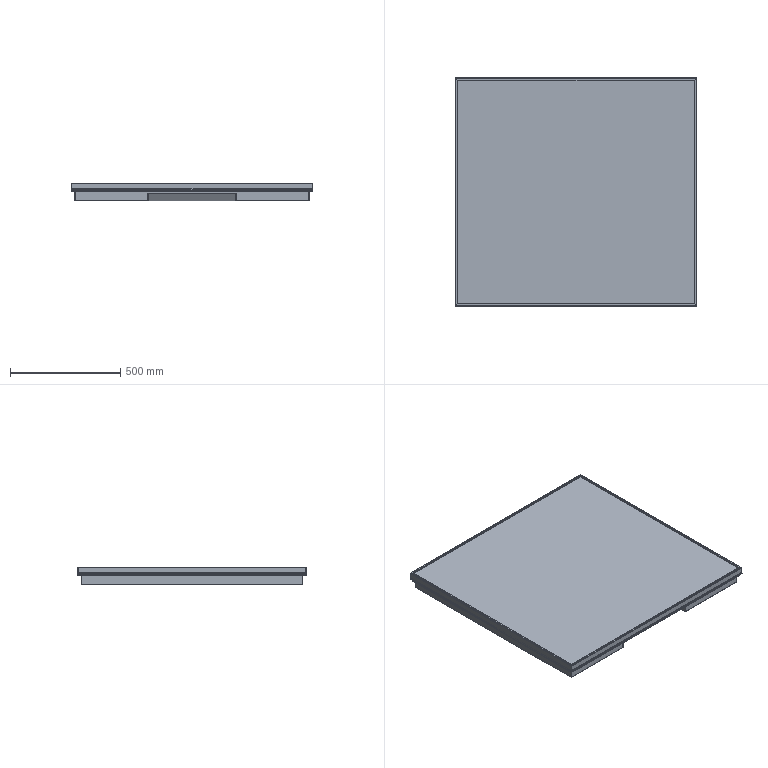Part | SolidWorks | 7 solids | 264 faces | box 1095 x 1035 x 80 mm | volume 5243599 mm3 | plane 176 | cylinder 76 | spline 12 | commonest cylinder face diameters 7 x30 11 x16 0.4 x9 2.4 x9 2 x6 1 x4